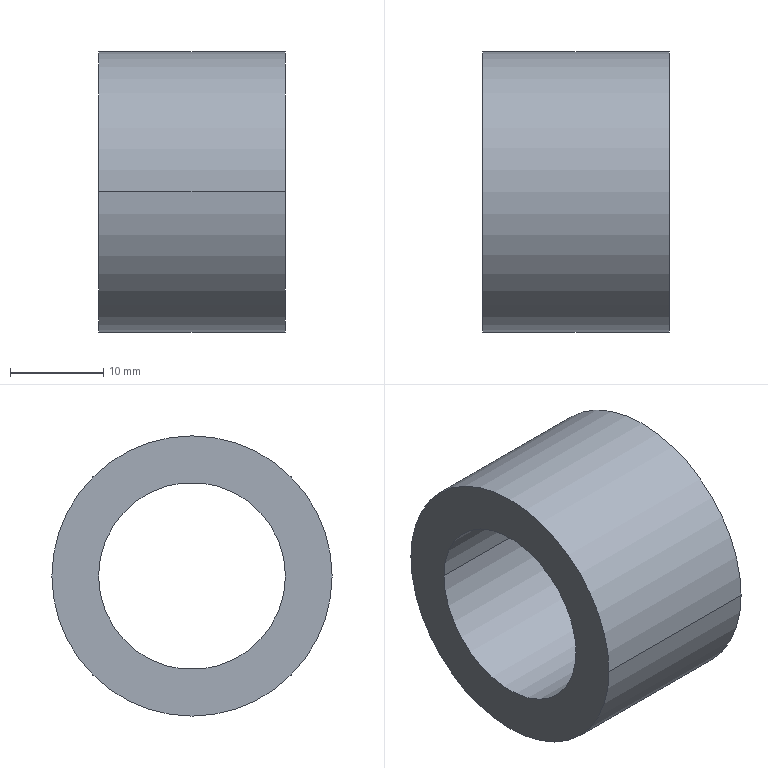Part | STEP file | P-008247^LM06S-05-06B | 1 solid | 6 faces | box 20 x 30 x 30 mm | volume 7854 mm3 | cylinder 4 | plane 2 | commonest cylinder face diameters 20 x2 30 x2
STEP:
#1=CARTESIAN_POINT('',(0.,0.,0.));
#2=DIRECTION('',(0.,0.,1.));
#3=DIRECTION('',(1.,0.,0.));
#4=AXIS2_PLACEMENT_3D('',#1,#2,#3);
#5=CARTESIAN_POINT('',(-10.,10.,0.));
#6=VERTEX_POINT('',#5);
#7=CARTESIAN_POINT('',(-10.,-10.,0.));
#8=VERTEX_POINT('',#7);
#9=CARTESIAN_POINT('',(-10.,0.,0.));
#10=DIRECTION('',(-1.,0.,0.));
#11=DIRECTION('',(0.,1.,0.));
#12=AXIS2_PLACEMENT_3D('',#9,#10,#11);
#13=CIRCLE('',#12,10.);
#14=CARTESIAN_POINT('',(-10.,0.,0.));
#15=DIRECTION('',(1.,0.,0.));
#16=DIRECTION('',(0.,1.,0.));
#17=AXIS2_PLACEMENT_3D('',#14,#15,#16);
#18=PLANE('',#17);
#19=CARTESIAN_POINT('',(10.,0.));
#20=CARTESIAN_POINT('',(10.,-17.321));
#21=CARTESIAN_POINT('',(-5.,-8.66));
#22=CARTESIAN_POINT('',(-20.,0.));
#23=CARTESIAN_POINT('',(-5.,8.66));
#24=CARTESIAN_POINT('',(10.,17.321));
#25=CARTESIAN_POINT('',(10.,0.));
#26=(BOUNDED_CURVE()B_SPLINE_CURVE(2,(#19,#20,#21,#22,#23,#24,#25),.UNSPECIFIED.,.T.,.F.)B_SPLINE_CURVE_WITH_KNOTS((1,2,2,2,2,1),(-2.094,0.,2.094,4.189,6.283,8.378),.UNSPECIFIED.)CURVE()GEOMETRIC_REPRESENTATION_ITEM()RATIONAL_B_SPLINE_CURVE((1.,0.5,1.,0.5,1.,0.5,1.))REPRESENTATION_ITEM(''));
#27=(GEOMETRIC_REPRESENTATION_CONTEXT(2)PARAMETRIC_REPRESENTATION_CONTEXT()REPRESENTATION_CONTEXT('',''));
#28=DEFINITIONAL_REPRESENTATION('',(#26),#27);
#29=PCURVE('',#18,#28);
#30=CARTESIAN_POINT('',(-10.,0.,0.));
#31=DIRECTION('',(1.,0.,0.));
#32=DIRECTION('',(0.,1.,0.));
#33=AXIS2_PLACEMENT_3D('',#30,#31,#32);
#34=CYLINDRICAL_SURFACE('',#33,10.);
#35=CARTESIAN_POINT('',(6.283,0.));
#36=DIRECTION('',(-1.,0.));
#37=VECTOR('',#36,1.);
#38=LINE('',#35,#37);
#39=(GEOMETRIC_REPRESENTATION_CONTEXT(2)PARAMETRIC_REPRESENTATION_CONTEXT()REPRESENTATION_CONTEXT('',''));
#40=DEFINITIONAL_REPRESENTATION('',(#38),#39);
#41=PCURVE('',#34,#40);
#42=SURFACE_CURVE('',#13,(#29,#41),.PCURVE_S1.);
#43=EDGE_CURVE('',#6,#8,#42,.T.);
#44=ORIENTED_EDGE('',*,*,#43,.F.);
#45=CARTESIAN_POINT('',(-10.,0.,0.));
#46=DIRECTION('',(-1.,0.,0.));
#47=DIRECTION('',(0.,1.,0.));
#48=AXIS2_PLACEMENT_3D('',#45,#46,#47);
#49=CIRCLE('',#48,10.);
#50=CARTESIAN_POINT('',(10.,0.));
#51=CARTESIAN_POINT('',(10.,-17.321));
#52=CARTESIAN_POINT('',(-5.,-8.66));
#53=CARTESIAN_POINT('',(-20.,0.));
#54=CARTESIAN_POINT('',(-5.,8.66));
#55=CARTESIAN_POINT('',(10.,17.321));
#56=CARTESIAN_POINT('',(10.,0.));
#57=(BOUNDED_CURVE()B_SPLINE_CURVE(2,(#50,#51,#52,#53,#54,#55,#56),.UNSPECIFIED.,.T.,.F.)B_SPLINE_CURVE_WITH_KNOTS((1,2,2,2,2,1),(-2.094,0.,2.094,4.189,6.283,8.378),.UNSPECIFIED.)CURVE()GEOMETRIC_REPRESENTATION_ITEM()RATIONAL_B_SPLINE_CURVE((1.,0.5,1.,0.5,1.,0.5,1.))REPRESENTATION_ITEM(''));
#58=(GEOMETRIC_REPRESENTATION_CONTEXT(2)PARAMETRIC_REPRESENTATION_CONTEXT()REPRESENTATION_CONTEXT('',''));
#59=DEFINITIONAL_REPRESENTATION('',(#57),#58);
#60=PCURVE('',#18,#59);
#61=CARTESIAN_POINT('',(-10.,0.,0.));
#62=DIRECTION('',(1.,0.,0.));
#63=DIRECTION('',(0.,1.,0.));
#64=AXIS2_PLACEMENT_3D('',#61,#62,#63);
#65=CYLINDRICAL_SURFACE('',#64,10.);
#66=CARTESIAN_POINT('',(6.283,0.));
#67=DIRECTION('',(-1.,0.));
#68=VECTOR('',#67,1.);
#69=LINE('',#66,#68);
#70=(GEOMETRIC_REPRESENTATION_CONTEXT(2)PARAMETRIC_REPRESENTATION_CONTEXT()REPRESENTATION_CONTEXT('',''));
#71=DEFINITIONAL_REPRESENTATION('',(#69),#70);
#72=PCURVE('',#65,#71);
#73=SURFACE_CURVE('',#49,(#60,#72),.PCURVE_S1.);
#74=EDGE_CURVE('',#8,#6,#73,.T.);
#75=ORIENTED_EDGE('',*,*,#74,.F.);
#76=EDGE_LOOP('',(#44,#75));
#77=FACE_BOUND('',#76,.T.);
#78=CARTESIAN_POINT('',(-10.,15.,0.));
#79=VERTEX_POINT('',#78);
#80=CARTESIAN_POINT('',(-10.,-15.,0.));
#81=VERTEX_POINT('',#80);
#82=CARTESIAN_POINT('',(-10.,0.,0.));
#83=DIRECTION('',(1.,0.,0.));
#84=DIRECTION('',(0.,1.,0.));
#85=AXIS2_PLACEMENT_3D('',#82,#83,#84);
#86=CIRCLE('',#85,15.);
#87=CARTESIAN_POINT('',(0.,0.));
#88=DIRECTION('',(1.,0.));
#89=AXIS2_PLACEMENT_2D('',#87,#88);
#90=CIRCLE('',#89,15.);
#91=(GEOMETRIC_REPRESENTATION_CONTEXT(2)PARAMETRIC_REPRESENTATION_CONTEXT()REPRESENTATION_CONTEXT('',''));
#92=DEFINITIONAL_REPRESENTATION('',(#90),#91);
#93=PCURVE('',#18,#92);
#94=CARTESIAN_POINT('',(-10.,0.,0.));
#95=DIRECTION('',(1.,0.,0.));
#96=DIRECTION('',(0.,1.,0.));
#97=AXIS2_PLACEMENT_3D('',#94,#95,#96);
#98=CYLINDRICAL_SURFACE('',#97,15.);
#99=CARTESIAN_POINT('',(0.,0.));
#100=DIRECTION('',(1.,0.));
#101=VECTOR('',#100,1.);
#102=LINE('',#99,#101);
#103=(GEOMETRIC_REPRESENTATION_CONTEXT(2)PARAMETRIC_REPRESENTATION_CONTEXT()REPRESENTATION_CONTEXT('',''));
#104=DEFINITIONAL_REPRESENTATION('',(#102),#103);
#105=PCURVE('',#98,#104);
#106=SURFACE_CURVE('',#86,(#93,#105),.PCURVE_S1.);
#107=EDGE_CURVE('',#79,#81,#106,.T.);
#108=ORIENTED_EDGE('',*,*,#107,.F.);
#109=CARTESIAN_POINT('',(-10.,0.,0.));
#110=DIRECTION('',(1.,0.,0.));
#111=DIRECTION('',(0.,1.,0.));
#112=AXIS2_PLACEMENT_3D('',#109,#110,#111);
#113=CIRCLE('',#112,15.);
#114=CARTESIAN_POINT('',(0.,0.));
#115=DIRECTION('',(1.,0.));
#116=AXIS2_PLACEMENT_2D('',#114,#115);
#117=CIRCLE('',#116,15.);
#118=(GEOMETRIC_REPRESENTATION_CONTEXT(2)PARAMETRIC_REPRESENTATION_CONTEXT()REPRESENTATION_CONTEXT('',''));
#119=DEFINITIONAL_REPRESENTATION('',(#117),#118);
#120=PCURVE('',#18,#119);
#121=CARTESIAN_POINT('',(-10.,0.,0.));
#122=DIRECTION('',(1.,0.,0.));
#123=DIRECTION('',(0.,1.,0.));
#124=AXIS2_PLACEMENT_3D('',#121,#122,#123);
#125=CYLINDRICAL_SURFACE('',#124,15.);
#126=CARTESIAN_POINT('',(0.,0.));
#127=DIRECTION('',(1.,0.));
#128=VECTOR('',#127,1.);
#129=LINE('',#126,#128);
#130=(GEOMETRIC_REPRESENTATION_CONTEXT(2)PARAMETRIC_REPRESENTATION_CONTEXT()REPRESENTATION_CONTEXT('',''));
#131=DEFINITIONAL_REPRESENTATION('',(#129),#130);
#132=PCURVE('',#125,#131);
#133=SURFACE_CURVE('',#113,(#120,#132),.PCURVE_S1.);
#134=EDGE_CURVE('',#81,#79,#133,.T.);
#135=ORIENTED_EDGE('',*,*,#134,.F.);
#136=EDGE_LOOP('',(#108,#135));
#137=FACE_BOUND('',#136,.T.);
#138=ADVANCED_FACE('',(#77,#137),#18,.F.);
#139=CARTESIAN_POINT('',(10.,10.,0.));
#140=VERTEX_POINT('',#139);
#141=CARTESIAN_POINT('',(10.,-10.,0.));
#142=VERTEX_POINT('',#141);
#143=CARTESIAN_POINT('',(10.,0.,0.));
#144=DIRECTION('',(1.,0.,0.));
#145=DIRECTION('',(0.,1.,0.));
#146=AXIS2_PLACEMENT_3D('',#143,#144,#145);
#147=CIRCLE('',#146,10.);
#148=CARTESIAN_POINT('',(10.,0.,0.));
#149=DIRECTION('',(1.,0.,0.));
#150=DIRECTION('',(0.,1.,0.));
#151=AXIS2_PLACEMENT_3D('',#148,#149,#150);
#152=PLANE('',#151);
#153=CARTESIAN_POINT('',(0.,0.));
#154=DIRECTION('',(1.,0.));
#155=AXIS2_PLACEMENT_2D('',#153,#154);
#156=CIRCLE('',#155,10.);
#157=(GEOMETRIC_REPRESENTATION_CONTEXT(2)PARAMETRIC_REPRESENTATION_CONTEXT()REPRESENTATION_CONTEXT('',''));
#158=DEFINITIONAL_REPRESENTATION('',(#156),#157);
#159=PCURVE('',#152,#158);
#160=CARTESIAN_POINT('',(0.,20.));
#161=DIRECTION('',(1.,0.));
#162=VECTOR('',#161,1.);
#163=LINE('',#160,#162);
#164=(GEOMETRIC_REPRESENTATION_CONTEXT(2)PARAMETRIC_REPRESENTATION_CONTEXT()REPRESENTATION_CONTEXT('',''));
#165=DEFINITIONAL_REPRESENTATION('',(#163),#164);
#166=PCURVE('',#65,#165);
#167=SURFACE_CURVE('',#147,(#159,#166),.PCURVE_S1.);
#168=EDGE_CURVE('',#140,#142,#167,.T.);
#169=ORIENTED_EDGE('',*,*,#168,.F.);
#170=CARTESIAN_POINT('',(10.,0.,0.));
#171=DIRECTION('',(1.,0.,0.));
#172=DIRECTION('',(0.,1.,0.));
#173=AXIS2_PLACEMENT_3D('',#170,#171,#172);
#174=CIRCLE('',#173,10.);
#175=CARTESIAN_POINT('',(0.,0.));
#176=DIRECTION('',(1.,0.));
#177=AXIS2_PLACEMENT_2D('',#175,#176);
#178=CIRCLE('',#177,10.);
#179=(GEOMETRIC_REPRESENTATION_CONTEXT(2)PARAMETRIC_REPRESENTATION_CONTEXT()REPRESENTATION_CONTEXT('',''));
#180=DEFINITIONAL_REPRESENTATION('',(#178),#179);
#181=PCURVE('',#152,#180);
#182=CARTESIAN_POINT('',(0.,20.));
#183=DIRECTION('',(1.,0.));
#184=VECTOR('',#183,1.);
#185=LINE('',#182,#184);
#186=(GEOMETRIC_REPRESENTATION_CONTEXT(2)PARAMETRIC_REPRESENTATION_CONTEXT()REPRESENTATION_CONTEXT('',''));
#187=DEFINITIONAL_REPRESENTATION('',(#185),#186);
#188=PCURVE('',#34,#187);
#189=SURFACE_CURVE('',#174,(#181,#188),.PCURVE_S1.);
#190=EDGE_CURVE('',#142,#140,#189,.T.);
#191=ORIENTED_EDGE('',*,*,#190,.F.);
#192=EDGE_LOOP('',(#169,#191));
#193=FACE_BOUND('',#192,.T.);
#194=CARTESIAN_POINT('',(10.,15.,0.));
#195=VERTEX_POINT('',#194);
#196=CARTESIAN_POINT('',(10.,-15.,0.));
#197=VERTEX_POINT('',#196);
#198=CARTESIAN_POINT('',(10.,0.,0.));
#199=DIRECTION('',(-1.,0.,0.));
#200=DIRECTION('',(0.,1.,0.));
#201=AXIS2_PLACEMENT_3D('',#198,#199,#200);
#202=CIRCLE('',#201,15.);
#203=CARTESIAN_POINT('',(15.,0.));
#204=CARTESIAN_POINT('',(15.,-25.981));
#205=CARTESIAN_POINT('',(-7.5,-12.99));
#206=CARTESIAN_POINT('',(-30.,0.));
#207=CARTESIAN_POINT('',(-7.5,12.99));
#208=CARTESIAN_POINT('',(15.,25.981));
#209=CARTESIAN_POINT('',(15.,0.));
#210=(BOUNDED_CURVE()B_SPLINE_CURVE(2,(#203,#204,#205,#206,#207,#208,#209),.UNSPECIFIED.,.T.,.F.)B_SPLINE_CURVE_WITH_KNOTS((1,2,2,2,2,1),(-2.094,0.,2.094,4.189,6.283,8.378),.UNSPECIFIED.)CURVE()GEOMETRIC_REPRESENTATION_ITEM()RATIONAL_B_SPLINE_CURVE((1.,0.5,1.,0.5,1.,0.5,1.))REPRESENTATION_ITEM(''));
#211=(GEOMETRIC_REPRESENTATION_CONTEXT(2)PARAMETRIC_REPRESENTATION_CONTEXT()REPRESENTATION_CONTEXT('',''));
#212=DEFINITIONAL_REPRESENTATION('',(#210),#211);
#213=PCURVE('',#152,#212);
#214=CARTESIAN_POINT('',(6.283,20.));
#215=DIRECTION('',(-1.,0.));
#216=VECTOR('',#215,1.);
#217=LINE('',#214,#216);
#218=(GEOMETRIC_REPRESENTATION_CONTEXT(2)PARAMETRIC_REPRESENTATION_CONTEXT()REPRESENTATION_CONTEXT('',''));
#219=DEFINITIONAL_REPRESENTATION('',(#217),#218);
#220=PCURVE('',#125,#219);
#221=SURFACE_CURVE('',#202,(#213,#220),.PCURVE_S1.);
#222=EDGE_CURVE('',#195,#197,#221,.T.);
#223=ORIENTED_EDGE('',*,*,#222,.F.);
#224=CARTESIAN_POINT('',(10.,0.,0.));
#225=DIRECTION('',(-1.,0.,0.));
#226=DIRECTION('',(0.,1.,0.));
#227=AXIS2_PLACEMENT_3D('',#224,#225,#226);
#228=CIRCLE('',#227,15.);
#229=CARTESIAN_POINT('',(15.,0.));
#230=CARTESIAN_POINT('',(15.,-25.981));
#231=CARTESIAN_POINT('',(-7.5,-12.99));
#232=CARTESIAN_POINT('',(-30.,0.));
#233=CARTESIAN_POINT('',(-7.5,12.99));
#234=CARTESIAN_POINT('',(15.,25.981));
#235=CARTESIAN_POINT('',(15.,0.));
#236=(BOUNDED_CURVE()B_SPLINE_CURVE(2,(#229,#230,#231,#232,#233,#234,#235),.UNSPECIFIED.,.T.,.F.)B_SPLINE_CURVE_WITH_KNOTS((1,2,2,2,2,1),(-2.094,0.,2.094,4.189,6.283,8.378),.UNSPECIFIED.)CURVE()GEOMETRIC_REPRESENTATION_ITEM()RATIONAL_B_SPLINE_CURVE((1.,0.5,1.,0.5,1.,0.5,1.))REPRESENTATION_ITEM(''));
#237=(GEOMETRIC_REPRESENTATION_CONTEXT(2)PARAMETRIC_REPRESENTATION_CONTEXT()REPRESENTATION_CONTEXT('',''));
#238=DEFINITIONAL_REPRESENTATION('',(#236),#237);
#239=PCURVE('',#152,#238);
#240=CARTESIAN_POINT('',(6.283,20.));
#241=DIRECTION('',(-1.,0.));
#242=VECTOR('',#241,1.);
#243=LINE('',#240,#242);
#244=(GEOMETRIC_REPRESENTATION_CONTEXT(2)PARAMETRIC_REPRESENTATION_CONTEXT()REPRESENTATION_CONTEXT('',''));
#245=DEFINITIONAL_REPRESENTATION('',(#243),#244);
#246=PCURVE('',#98,#245);
#247=SURFACE_CURVE('',#228,(#239,#246),.PCURVE_S1.);
#248=EDGE_CURVE('',#197,#195,#247,.T.);
#249=ORIENTED_EDGE('',*,*,#248,.F.);
#250=EDGE_LOOP('',(#223,#249));
#251=FACE_BOUND('',#250,.T.);
#252=ADVANCED_FACE('',(#193,#251),#152,.T.);
#253=ORIENTED_EDGE('',*,*,#190,.F.);
#254=CARTESIAN_POINT('',(10.,-10.,0.));
#255=DIRECTION('',(-1.,0.,0.));
#256=VECTOR('',#255,1.);
#257=LINE('',#254,#256);
#258=CARTESIAN_POINT('',(3.142,20.));
#259=DIRECTION('',(0.,-1.));
#260=VECTOR('',#259,1.);
#261=LINE('',#258,#260);
#262=(GEOMETRIC_REPRESENTATION_CONTEXT(2)PARAMETRIC_REPRESENTATION_CONTEXT()REPRESENTATION_CONTEXT('',''));
#263=DEFINITIONAL_REPRESENTATION('',(#261),#262);
#264=PCURVE('',#34,#263);
#265=CARTESIAN_POINT('',(3.142,20.));
#266=DIRECTION('',(0.,-1.));
#267=VECTOR('',#266,1.);
#268=LINE('',#265,#267);
#269=(GEOMETRIC_REPRESENTATION_CONTEXT(2)PARAMETRIC_REPRESENTATION_CONTEXT()REPRESENTATION_CONTEXT('',''));
#270=DEFINITIONAL_REPRESENTATION('',(#268),#269);
#271=PCURVE('',#65,#270);
#272=SURFACE_CURVE('',#257,(#264,#271),.PCURVE_S1.);
#273=EDGE_CURVE('',#142,#8,#272,.T.);
#274=ORIENTED_EDGE('',*,*,#273,.T.);
#275=ORIENTED_EDGE('',*,*,#43,.F.);
#276=CARTESIAN_POINT('',(10.,10.,0.));
#277=DIRECTION('',(-1.,0.,0.));
#278=VECTOR('',#277,1.);
#279=LINE('',#276,#278);
#280=CARTESIAN_POINT('',(6.283,20.));
#281=DIRECTION('',(0.,-1.));
#282=VECTOR('',#281,1.);
#283=LINE('',#280,#282);
#284=(GEOMETRIC_REPRESENTATION_CONTEXT(2)PARAMETRIC_REPRESENTATION_CONTEXT()REPRESENTATION_CONTEXT('',''));
#285=DEFINITIONAL_REPRESENTATION('',(#283),#284);
#286=PCURVE('',#34,#285);
#287=CARTESIAN_POINT('',(0.,20.));
#288=DIRECTION('',(0.,-1.));
#289=VECTOR('',#288,1.);
#290=LINE('',#287,#289);
#291=(GEOMETRIC_REPRESENTATION_CONTEXT(2)PARAMETRIC_REPRESENTATION_CONTEXT()REPRESENTATION_CONTEXT('',''));
#292=DEFINITIONAL_REPRESENTATION('',(#290),#291);
#293=PCURVE('',#65,#292);
#294=SURFACE_CURVE('',#279,(#286,#293),.PCURVE_S1.);
#295=EDGE_CURVE('',#140,#6,#294,.T.);
#296=ORIENTED_EDGE('',*,*,#295,.F.);
#297=EDGE_LOOP('',(#253,#274,#275,#296));
#298=FACE_BOUND('',#297,.F.);
#299=ADVANCED_FACE('',(#298),#34,.F.);
#300=CARTESIAN_POINT('',(10.,15.,0.));
#301=DIRECTION('',(-1.,0.,0.));
#302=VECTOR('',#301,1.);
#303=LINE('',#300,#302);
#304=CARTESIAN_POINT('',(0.,20.));
#305=DIRECTION('',(0.,-1.));
#306=VECTOR('',#305,1.);
#307=LINE('',#304,#306);
#308=(GEOMETRIC_REPRESENTATION_CONTEXT(2)PARAMETRIC_REPRESENTATION_CONTEXT()REPRESENTATION_CONTEXT('',''));
#309=DEFINITIONAL_REPRESENTATION('',(#307),#308);
#310=PCURVE('',#98,#309);
#311=CARTESIAN_POINT('',(6.283,20.));
#312=DIRECTION('',(0.,-1.));
#313=VECTOR('',#312,1.);
#314=LINE('',#311,#313);
#315=(GEOMETRIC_REPRESENTATION_CONTEXT(2)PARAMETRIC_REPRESENTATION_CONTEXT()REPRESENTATION_CONTEXT('',''));
#316=DEFINITIONAL_REPRESENTATION('',(#314),#315);
#317=PCURVE('',#125,#316);
#318=SURFACE_CURVE('',#303,(#310,#317),.PCURVE_S1.);
#319=EDGE_CURVE('',#195,#79,#318,.T.);
#320=ORIENTED_EDGE('',*,*,#319,.T.);
#321=ORIENTED_EDGE('',*,*,#107,.T.);
#322=CARTESIAN_POINT('',(10.,-15.,0.));
#323=DIRECTION('',(-1.,0.,0.));
#324=VECTOR('',#323,1.);
#325=LINE('',#322,#324);
#326=CARTESIAN_POINT('',(3.142,20.));
#327=DIRECTION('',(0.,-1.));
#328=VECTOR('',#327,1.);
#329=LINE('',#326,#328);
#330=(GEOMETRIC_REPRESENTATION_CONTEXT(2)PARAMETRIC_REPRESENTATION_CONTEXT()REPRESENTATION_CONTEXT('',''));
#331=DEFINITIONAL_REPRESENTATION('',(#329),#330);
#332=PCURVE('',#98,#331);
#333=CARTESIAN_POINT('',(3.142,20.));
#334=DIRECTION('',(0.,-1.));
#335=VECTOR('',#334,1.);
#336=LINE('',#333,#335);
#337=(GEOMETRIC_REPRESENTATION_CONTEXT(2)PARAMETRIC_REPRESENTATION_CONTEXT()REPRESENTATION_CONTEXT('',''));
#338=DEFINITIONAL_REPRESENTATION('',(#336),#337);
#339=PCURVE('',#125,#338);
#340=SURFACE_CURVE('',#325,(#332,#339),.PCURVE_S1.);
#341=EDGE_CURVE('',#197,#81,#340,.T.);
#342=ORIENTED_EDGE('',*,*,#341,.F.);
#343=ORIENTED_EDGE('',*,*,#248,.T.);
#344=EDGE_LOOP('',(#320,#321,#342,#343));
#345=FACE_BOUND('',#344,.T.);
#346=ADVANCED_FACE('',(#345),#98,.T.);
#347=ORIENTED_EDGE('',*,*,#319,.F.);
#348=ORIENTED_EDGE('',*,*,#222,.T.);
#349=ORIENTED_EDGE('',*,*,#341,.T.);
#350=ORIENTED_EDGE('',*,*,#134,.T.);
#351=EDGE_LOOP('',(#347,#348,#349,#350));
#352=FACE_BOUND('',#351,.T.);
#353=ADVANCED_FACE('',(#352),#125,.T.);
#354=ORIENTED_EDGE('',*,*,#74,.F.);
#355=ORIENTED_EDGE('',*,*,#273,.F.);
#356=ORIENTED_EDGE('',*,*,#168,.F.);
#357=ORIENTED_EDGE('',*,*,#295,.T.);
#358=EDGE_LOOP('',(#354,#355,#356,#357));
#359=FACE_BOUND('',#358,.F.);
#360=ADVANCED_FACE('',(#359),#65,.F.);
#361=CLOSED_SHELL('',(#138,#252,#299,#346,#353,#360));
#362=MANIFOLD_SOLID_BREP('',#361);
#363=(LENGTH_UNIT()NAMED_UNIT(*)SI_UNIT(.MILLI.,.METRE.));
#364=UNCERTAINTY_MEASURE_WITH_UNIT(LENGTH_MEASURE(0.0000001),#363,'','');
#365=(NAMED_UNIT(*)PLANE_ANGLE_UNIT()SI_UNIT($,.RADIAN.));
#366=(NAMED_UNIT(*)SI_UNIT($,.STERADIAN.)SOLID_ANGLE_UNIT());
#367=(GEOMETRIC_REPRESENTATION_CONTEXT(3)GLOBAL_UNCERTAINTY_ASSIGNED_CONTEXT((#364))GLOBAL_UNIT_ASSIGNED_CONTEXT((#363,#365,#366))REPRESENTATION_CONTEXT('',''));
#368=ADVANCED_BREP_SHAPE_REPRESENTATION('',(#4,#362),#367);